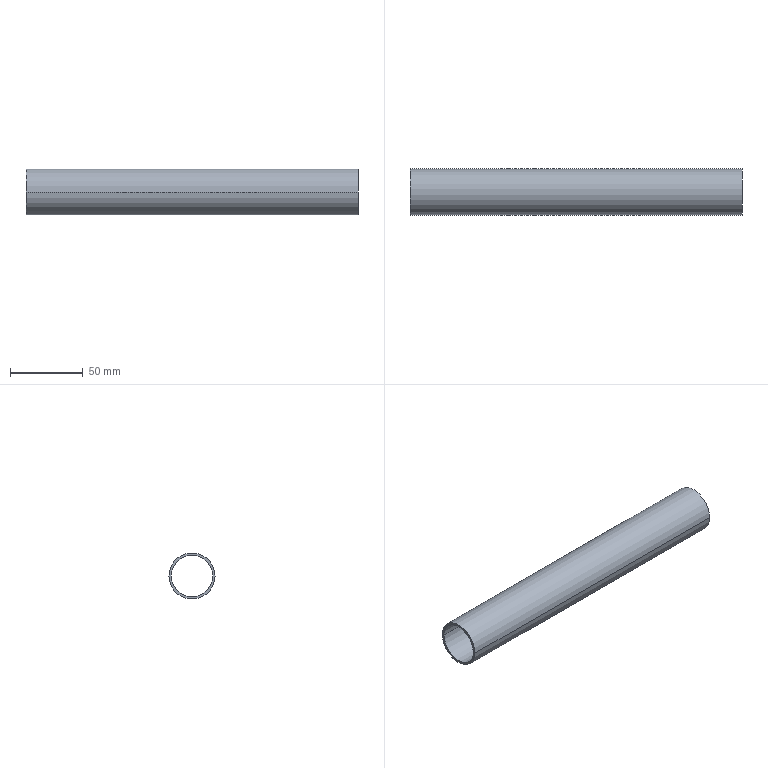Part | NX | features BREP 1 | 1 solid | 6 faces | box 228.6 x 31.75 x 31.75 mm | volume 34388 mm3 | cylinder 4 | plane 2 | commonest cylinder face diameters 28.575 x2 31.75 x2
STEP:
#1=CARTESIAN_POINT('',(-114.3,15.875,0.));
#2=VERTEX_POINT('',#1);
#3=CARTESIAN_POINT('',(-114.3,-15.875,0.));
#4=VERTEX_POINT('',#3);
#5=CARTESIAN_POINT('',(-114.3,0.,0.));
#6=DIRECTION('',(1.,0.,0.));
#7=DIRECTION('',(0.,1.,0.));
#8=AXIS2_PLACEMENT_3D('',#5,#6,#7);
#9=CIRCLE('',#8,15.875);
#10=EDGE_CURVE('',#2,#4,#9,.T.);
#11=ORIENTED_EDGE('',*,*,#10,.F.);
#12=CARTESIAN_POINT('',(-114.3,0.,0.));
#13=DIRECTION('',(1.,0.,0.));
#14=DIRECTION('',(0.,-1.,0.));
#15=AXIS2_PLACEMENT_3D('',#12,#13,#14);
#16=CIRCLE('',#15,15.875);
#17=EDGE_CURVE('',#4,#2,#16,.T.);
#18=ORIENTED_EDGE('',*,*,#17,.F.);
#19=EDGE_LOOP('',(#11,#18));
#20=FACE_BOUND('',#19,.T.);
#21=CARTESIAN_POINT('',(-114.3,14.287,0.));
#22=VERTEX_POINT('',#21);
#23=CARTESIAN_POINT('',(-114.3,-14.287,0.));
#24=VERTEX_POINT('',#23);
#25=CARTESIAN_POINT('',(-114.3,0.,0.));
#26=DIRECTION('',(-1.,0.,0.));
#27=DIRECTION('',(0.,1.,0.));
#28=AXIS2_PLACEMENT_3D('',#25,#26,#27);
#29=CIRCLE('',#28,14.287);
#30=EDGE_CURVE('',#22,#24,#29,.T.);
#31=ORIENTED_EDGE('',*,*,#30,.F.);
#32=CARTESIAN_POINT('',(-114.3,0.,0.));
#33=DIRECTION('',(-1.,0.,0.));
#34=DIRECTION('',(0.,-1.,0.));
#35=AXIS2_PLACEMENT_3D('',#32,#33,#34);
#36=CIRCLE('',#35,14.287);
#37=EDGE_CURVE('',#24,#22,#36,.T.);
#38=ORIENTED_EDGE('',*,*,#37,.F.);
#39=EDGE_LOOP('',(#31,#38));
#40=FACE_BOUND('',#39,.T.);
#41=CARTESIAN_POINT('',(-114.3,0.,0.));
#42=DIRECTION('',(1.,0.,0.));
#43=DIRECTION('',(0.,1.,0.));
#44=AXIS2_PLACEMENT_3D('',#41,#42,#43);
#45=PLANE('',#44);
#46=ADVANCED_FACE('',(#20,#40),#45,.F.);
#47=CARTESIAN_POINT('',(114.3,15.875,0.));
#48=VERTEX_POINT('',#47);
#49=CARTESIAN_POINT('',(-114.3,15.875,0.));
#50=DIRECTION('',(1.,0.,0.));
#51=VECTOR('',#50,1000.);
#52=LINE('',#49,#51);
#53=EDGE_CURVE('',#48,#2,#52,.F.);
#54=ORIENTED_EDGE('',*,*,#53,.F.);
#55=CARTESIAN_POINT('',(114.3,-15.875,0.));
#56=VERTEX_POINT('',#55);
#57=CARTESIAN_POINT('',(114.3,0.,0.));
#58=DIRECTION('',(1.,0.,0.));
#59=DIRECTION('',(0.,-1.,0.));
#60=AXIS2_PLACEMENT_3D('',#57,#58,#59);
#61=CIRCLE('',#60,15.875);
#62=EDGE_CURVE('',#56,#48,#61,.T.);
#63=ORIENTED_EDGE('',*,*,#62,.F.);
#64=CARTESIAN_POINT('',(-114.3,-15.875,0.));
#65=DIRECTION('',(1.,0.,0.));
#66=VECTOR('',#65,1000.);
#67=LINE('',#64,#66);
#68=EDGE_CURVE('',#56,#4,#67,.F.);
#69=ORIENTED_EDGE('',*,*,#68,.T.);
#70=ORIENTED_EDGE('',*,*,#17,.T.);
#71=EDGE_LOOP('',(#54,#63,#69,#70));
#72=FACE_BOUND('',#71,.T.);
#73=CARTESIAN_POINT('',(-114.3,0.,0.));
#74=DIRECTION('',(1.,0.,0.));
#75=DIRECTION('',(0.,-1.,0.));
#76=AXIS2_PLACEMENT_3D('',#73,#74,#75);
#77=CYLINDRICAL_SURFACE('',#76,15.875);
#78=ADVANCED_FACE('',(#72),#77,.T.);
#79=ORIENTED_EDGE('',*,*,#68,.F.);
#80=CARTESIAN_POINT('',(114.3,0.,0.));
#81=DIRECTION('',(1.,0.,0.));
#82=DIRECTION('',(0.,1.,0.));
#83=AXIS2_PLACEMENT_3D('',#80,#81,#82);
#84=CIRCLE('',#83,15.875);
#85=EDGE_CURVE('',#48,#56,#84,.T.);
#86=ORIENTED_EDGE('',*,*,#85,.F.);
#87=ORIENTED_EDGE('',*,*,#53,.T.);
#88=ORIENTED_EDGE('',*,*,#10,.T.);
#89=EDGE_LOOP('',(#79,#86,#87,#88));
#90=FACE_BOUND('',#89,.T.);
#91=CARTESIAN_POINT('',(-114.3,0.,0.));
#92=DIRECTION('',(1.,0.,0.));
#93=DIRECTION('',(0.,-1.,0.));
#94=AXIS2_PLACEMENT_3D('',#91,#92,#93);
#95=CYLINDRICAL_SURFACE('',#94,15.875);
#96=ADVANCED_FACE('',(#90),#95,.T.);
#97=ORIENTED_EDGE('',*,*,#85,.T.);
#98=ORIENTED_EDGE('',*,*,#62,.T.);
#99=EDGE_LOOP('',(#97,#98));
#100=FACE_BOUND('',#99,.T.);
#101=CARTESIAN_POINT('',(114.3,14.287,0.));
#102=VERTEX_POINT('',#101);
#103=CARTESIAN_POINT('',(114.3,-14.287,0.));
#104=VERTEX_POINT('',#103);
#105=CARTESIAN_POINT('',(114.3,0.,0.));
#106=DIRECTION('',(-1.,0.,0.));
#107=DIRECTION('',(0.,1.,0.));
#108=AXIS2_PLACEMENT_3D('',#105,#106,#107);
#109=CIRCLE('',#108,14.287);
#110=EDGE_CURVE('',#102,#104,#109,.T.);
#111=ORIENTED_EDGE('',*,*,#110,.T.);
#112=CARTESIAN_POINT('',(114.3,0.,0.));
#113=DIRECTION('',(-1.,0.,0.));
#114=DIRECTION('',(0.,-1.,0.));
#115=AXIS2_PLACEMENT_3D('',#112,#113,#114);
#116=CIRCLE('',#115,14.287);
#117=EDGE_CURVE('',#104,#102,#116,.T.);
#118=ORIENTED_EDGE('',*,*,#117,.T.);
#119=EDGE_LOOP('',(#111,#118));
#120=FACE_BOUND('',#119,.T.);
#121=CARTESIAN_POINT('',(114.3,0.,0.));
#122=DIRECTION('',(1.,0.,0.));
#123=DIRECTION('',(0.,1.,0.));
#124=AXIS2_PLACEMENT_3D('',#121,#122,#123);
#125=PLANE('',#124);
#126=ADVANCED_FACE('',(#100,#120),#125,.T.);
#127=CARTESIAN_POINT('',(-114.3,14.287,0.));
#128=DIRECTION('',(1.,0.,0.));
#129=VECTOR('',#128,1000.);
#130=LINE('',#127,#129);
#131=EDGE_CURVE('',#102,#22,#130,.F.);
#132=ORIENTED_EDGE('',*,*,#131,.F.);
#133=ORIENTED_EDGE('',*,*,#117,.F.);
#134=CARTESIAN_POINT('',(-114.3,-14.287,0.));
#135=DIRECTION('',(1.,0.,0.));
#136=VECTOR('',#135,1000.);
#137=LINE('',#134,#136);
#138=EDGE_CURVE('',#104,#24,#137,.F.);
#139=ORIENTED_EDGE('',*,*,#138,.T.);
#140=ORIENTED_EDGE('',*,*,#37,.T.);
#141=EDGE_LOOP('',(#132,#133,#139,#140));
#142=FACE_BOUND('',#141,.T.);
#143=CARTESIAN_POINT('',(-114.3,0.,0.));
#144=DIRECTION('',(1.,0.,0.));
#145=DIRECTION('',(0.,-1.,0.));
#146=AXIS2_PLACEMENT_3D('',#143,#144,#145);
#147=CYLINDRICAL_SURFACE('',#146,14.287);
#148=ADVANCED_FACE('',(#142),#147,.F.);
#149=ORIENTED_EDGE('',*,*,#138,.F.);
#150=ORIENTED_EDGE('',*,*,#110,.F.);
#151=ORIENTED_EDGE('',*,*,#131,.T.);
#152=ORIENTED_EDGE('',*,*,#30,.T.);
#153=EDGE_LOOP('',(#149,#150,#151,#152));
#154=FACE_BOUND('',#153,.T.);
#155=CARTESIAN_POINT('',(-114.3,0.,0.));
#156=DIRECTION('',(1.,0.,0.));
#157=DIRECTION('',(0.,-1.,0.));
#158=AXIS2_PLACEMENT_3D('',#155,#156,#157);
#159=CYLINDRICAL_SURFACE('',#158,14.287);
#160=ADVANCED_FACE('',(#154),#159,.F.);
#161=CLOSED_SHELL('',(#46,#78,#96,#126,#148,#160));
#162=MANIFOLD_SOLID_BREP('',#161);
#163=(LENGTH_UNIT()NAMED_UNIT(*)SI_UNIT(.MILLI.,.METRE.));
#164=UNCERTAINTY_MEASURE_WITH_UNIT(LENGTH_MEASURE(0.00001),#163,'','');
#165=(NAMED_UNIT(*)PLANE_ANGLE_UNIT()SI_UNIT($,.RADIAN.));
#166=(NAMED_UNIT(*)SI_UNIT($,.STERADIAN.)SOLID_ANGLE_UNIT());
#167=(GEOMETRIC_REPRESENTATION_CONTEXT(3)GLOBAL_UNCERTAINTY_ASSIGNED_CONTEXT((#164))GLOBAL_UNIT_ASSIGNED_CONTEXT((#163,#165,#166))REPRESENTATION_CONTEXT('',''));
#168=ADVANCED_BREP_SHAPE_REPRESENTATION('',(#162),#167);